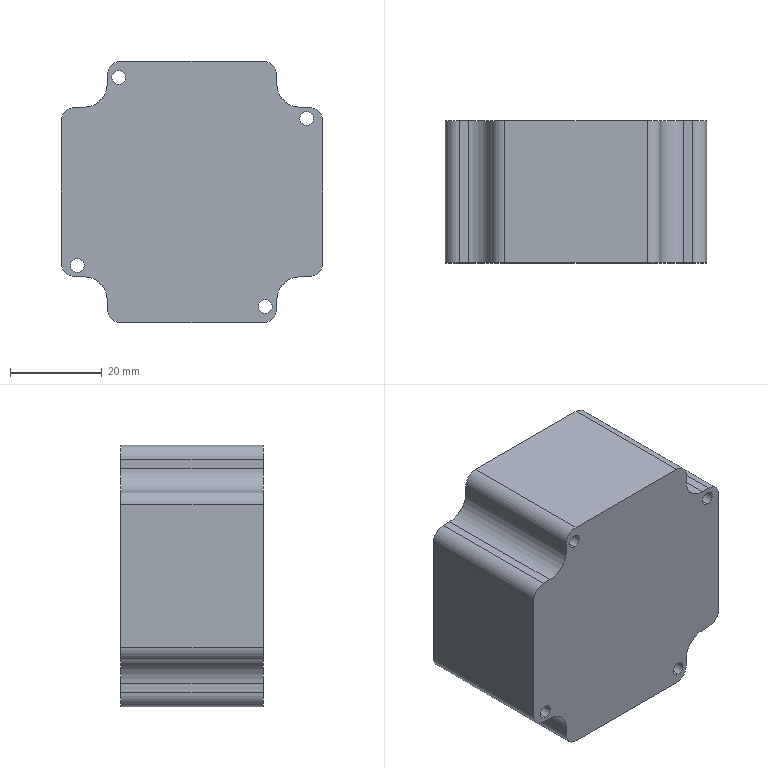Part | SolidWorks | features BaseBody 1 | 1 solid | 34 faces | box 57 x 31 x 57 mm | volume 87629 mm3 | cylinder 20 | plane 14 | commonest cylinder face diameters 3 x8 6 x8 10 x4
STEP:
#1=CARTESIAN_POINT('',(-16.,0.,23.5));
#2=VERTEX_POINT('',#1);
#3=CARTESIAN_POINT('',(-16.,0.,26.5));
#4=VERTEX_POINT('',#3);
#5=CARTESIAN_POINT('',(-16.,0.,25.));
#6=DIRECTION('',(0.,1.,0.));
#7=DIRECTION('',(0.,0.,1.));
#8=AXIS2_PLACEMENT_3D('',#5,#6,#7);
#9=CIRCLE('',#8,1.5);
#10=EDGE_CURVE('',#2,#4,#9,.T.);
#11=ORIENTED_EDGE('',*,*,#10,.F.);
#12=CARTESIAN_POINT('',(-16.,31.,23.5));
#13=VERTEX_POINT('',#12);
#14=CARTESIAN_POINT('',(-16.,0.,23.5));
#15=DIRECTION('',(0.,1.,0.));
#16=VECTOR('',#15,1000.);
#17=LINE('',#14,#16);
#18=EDGE_CURVE('',#2,#13,#17,.T.);
#19=ORIENTED_EDGE('',*,*,#18,.T.);
#20=CARTESIAN_POINT('',(-16.,31.,26.5));
#21=VERTEX_POINT('',#20);
#22=CARTESIAN_POINT('',(-16.,31.,25.));
#23=DIRECTION('',(0.,1.,0.));
#24=DIRECTION('',(0.,0.,1.));
#25=AXIS2_PLACEMENT_3D('',#22,#23,#24);
#26=CIRCLE('',#25,1.5);
#27=EDGE_CURVE('',#13,#21,#26,.T.);
#28=ORIENTED_EDGE('',*,*,#27,.T.);
#29=CARTESIAN_POINT('',(-16.,0.,26.5));
#30=DIRECTION('',(0.,1.,0.));
#31=VECTOR('',#30,1000.);
#32=LINE('',#29,#31);
#33=EDGE_CURVE('',#4,#21,#32,.T.);
#34=ORIENTED_EDGE('',*,*,#33,.F.);
#35=EDGE_LOOP('',(#11,#19,#28,#34));
#36=FACE_OUTER_BOUND('',#35,.T.);
#37=CARTESIAN_POINT('',(-16.,0.,25.));
#38=DIRECTION('',(0.,1.,0.));
#39=DIRECTION('',(0.,0.,1.));
#40=AXIS2_PLACEMENT_3D('',#37,#38,#39);
#41=CYLINDRICAL_SURFACE('',#40,1.5);
#42=ADVANCED_FACE('',(#36),#41,.F.);
#43=CARTESIAN_POINT('',(-25.,0.,-17.5));
#44=VERTEX_POINT('',#43);
#45=CARTESIAN_POINT('',(-25.,0.,-14.5));
#46=VERTEX_POINT('',#45);
#47=CARTESIAN_POINT('',(-25.,0.,-16.));
#48=DIRECTION('',(0.,1.,0.));
#49=DIRECTION('',(0.,0.,1.));
#50=AXIS2_PLACEMENT_3D('',#47,#48,#49);
#51=CIRCLE('',#50,1.5);
#52=EDGE_CURVE('',#44,#46,#51,.T.);
#53=ORIENTED_EDGE('',*,*,#52,.F.);
#54=CARTESIAN_POINT('',(-25.,31.,-17.5));
#55=VERTEX_POINT('',#54);
#56=CARTESIAN_POINT('',(-25.,0.,-17.5));
#57=DIRECTION('',(0.,1.,0.));
#58=VECTOR('',#57,1000.);
#59=LINE('',#56,#58);
#60=EDGE_CURVE('',#44,#55,#59,.T.);
#61=ORIENTED_EDGE('',*,*,#60,.T.);
#62=CARTESIAN_POINT('',(-25.,31.,-14.5));
#63=VERTEX_POINT('',#62);
#64=CARTESIAN_POINT('',(-25.,31.,-16.));
#65=DIRECTION('',(0.,1.,0.));
#66=DIRECTION('',(0.,0.,1.));
#67=AXIS2_PLACEMENT_3D('',#64,#65,#66);
#68=CIRCLE('',#67,1.5);
#69=EDGE_CURVE('',#55,#63,#68,.T.);
#70=ORIENTED_EDGE('',*,*,#69,.T.);
#71=CARTESIAN_POINT('',(-25.,0.,-14.5));
#72=DIRECTION('',(0.,1.,0.));
#73=VECTOR('',#72,1000.);
#74=LINE('',#71,#73);
#75=EDGE_CURVE('',#46,#63,#74,.T.);
#76=ORIENTED_EDGE('',*,*,#75,.F.);
#77=EDGE_LOOP('',(#53,#61,#70,#76));
#78=FACE_OUTER_BOUND('',#77,.T.);
#79=CARTESIAN_POINT('',(-25.,0.,-16.));
#80=DIRECTION('',(0.,1.,0.));
#81=DIRECTION('',(0.,0.,1.));
#82=AXIS2_PLACEMENT_3D('',#79,#80,#81);
#83=CYLINDRICAL_SURFACE('',#82,1.5);
#84=ADVANCED_FACE('',(#78),#83,.F.);
#85=CARTESIAN_POINT('',(16.,0.,-26.5));
#86=VERTEX_POINT('',#85);
#87=CARTESIAN_POINT('',(16.,0.,-23.5));
#88=VERTEX_POINT('',#87);
#89=CARTESIAN_POINT('',(16.,0.,-25.));
#90=DIRECTION('',(0.,1.,0.));
#91=DIRECTION('',(0.,0.,1.));
#92=AXIS2_PLACEMENT_3D('',#89,#90,#91);
#93=CIRCLE('',#92,1.5);
#94=EDGE_CURVE('',#86,#88,#93,.T.);
#95=ORIENTED_EDGE('',*,*,#94,.F.);
#96=CARTESIAN_POINT('',(16.,31.,-26.5));
#97=VERTEX_POINT('',#96);
#98=CARTESIAN_POINT('',(16.,0.,-26.5));
#99=DIRECTION('',(0.,1.,0.));
#100=VECTOR('',#99,1000.);
#101=LINE('',#98,#100);
#102=EDGE_CURVE('',#86,#97,#101,.T.);
#103=ORIENTED_EDGE('',*,*,#102,.T.);
#104=CARTESIAN_POINT('',(16.,31.,-23.5));
#105=VERTEX_POINT('',#104);
#106=CARTESIAN_POINT('',(16.,31.,-25.));
#107=DIRECTION('',(0.,1.,0.));
#108=DIRECTION('',(0.,0.,1.));
#109=AXIS2_PLACEMENT_3D('',#106,#107,#108);
#110=CIRCLE('',#109,1.5);
#111=EDGE_CURVE('',#97,#105,#110,.T.);
#112=ORIENTED_EDGE('',*,*,#111,.T.);
#113=CARTESIAN_POINT('',(16.,0.,-23.5));
#114=DIRECTION('',(0.,1.,0.));
#115=VECTOR('',#114,1000.);
#116=LINE('',#113,#115);
#117=EDGE_CURVE('',#88,#105,#116,.T.);
#118=ORIENTED_EDGE('',*,*,#117,.F.);
#119=EDGE_LOOP('',(#95,#103,#112,#118));
#120=FACE_OUTER_BOUND('',#119,.T.);
#121=CARTESIAN_POINT('',(16.,0.,-25.));
#122=DIRECTION('',(0.,1.,0.));
#123=DIRECTION('',(0.,0.,1.));
#124=AXIS2_PLACEMENT_3D('',#121,#122,#123);
#125=CYLINDRICAL_SURFACE('',#124,1.5);
#126=ADVANCED_FACE('',(#120),#125,.F.);
#127=CARTESIAN_POINT('',(25.,0.,14.5));
#128=VERTEX_POINT('',#127);
#129=CARTESIAN_POINT('',(25.,0.,17.5));
#130=VERTEX_POINT('',#129);
#131=CARTESIAN_POINT('',(25.,0.,16.));
#132=DIRECTION('',(0.,1.,0.));
#133=DIRECTION('',(0.,0.,1.));
#134=AXIS2_PLACEMENT_3D('',#131,#132,#133);
#135=CIRCLE('',#134,1.5);
#136=EDGE_CURVE('',#128,#130,#135,.T.);
#137=ORIENTED_EDGE('',*,*,#136,.F.);
#138=CARTESIAN_POINT('',(25.,31.,14.5));
#139=VERTEX_POINT('',#138);
#140=CARTESIAN_POINT('',(25.,0.,14.5));
#141=DIRECTION('',(0.,1.,0.));
#142=VECTOR('',#141,1000.);
#143=LINE('',#140,#142);
#144=EDGE_CURVE('',#128,#139,#143,.T.);
#145=ORIENTED_EDGE('',*,*,#144,.T.);
#146=CARTESIAN_POINT('',(25.,31.,17.5));
#147=VERTEX_POINT('',#146);
#148=CARTESIAN_POINT('',(25.,31.,16.));
#149=DIRECTION('',(0.,1.,0.));
#150=DIRECTION('',(0.,0.,1.));
#151=AXIS2_PLACEMENT_3D('',#148,#149,#150);
#152=CIRCLE('',#151,1.5);
#153=EDGE_CURVE('',#139,#147,#152,.T.);
#154=ORIENTED_EDGE('',*,*,#153,.T.);
#155=CARTESIAN_POINT('',(25.,0.,17.5));
#156=DIRECTION('',(0.,1.,0.));
#157=VECTOR('',#156,1000.);
#158=LINE('',#155,#157);
#159=EDGE_CURVE('',#130,#147,#158,.T.);
#160=ORIENTED_EDGE('',*,*,#159,.F.);
#161=EDGE_LOOP('',(#137,#145,#154,#160));
#162=FACE_OUTER_BOUND('',#161,.T.);
#163=CARTESIAN_POINT('',(25.,0.,16.));
#164=DIRECTION('',(0.,1.,0.));
#165=DIRECTION('',(0.,0.,1.));
#166=AXIS2_PLACEMENT_3D('',#163,#164,#165);
#167=CYLINDRICAL_SURFACE('',#166,1.5);
#168=ADVANCED_FACE('',(#162),#167,.F.);
#169=CARTESIAN_POINT('',(-16.,31.,25.));
#170=DIRECTION('',(0.,1.,0.));
#171=DIRECTION('',(0.,0.,1.));
#172=AXIS2_PLACEMENT_3D('',#169,#170,#171);
#173=CIRCLE('',#172,1.5);
#174=EDGE_CURVE('',#21,#13,#173,.T.);
#175=ORIENTED_EDGE('',*,*,#174,.F.);
#176=ORIENTED_EDGE('',*,*,#27,.F.);
#177=EDGE_LOOP('',(#175,#176));
#178=FACE_BOUND('',#177,.T.);
#179=CARTESIAN_POINT('',(-25.,31.,-16.));
#180=DIRECTION('',(0.,1.,0.));
#181=DIRECTION('',(0.,0.,1.));
#182=AXIS2_PLACEMENT_3D('',#179,#180,#181);
#183=CIRCLE('',#182,1.5);
#184=EDGE_CURVE('',#63,#55,#183,.T.);
#185=ORIENTED_EDGE('',*,*,#184,.F.);
#186=ORIENTED_EDGE('',*,*,#69,.F.);
#187=EDGE_LOOP('',(#185,#186));
#188=FACE_BOUND('',#187,.T.);
#189=CARTESIAN_POINT('',(16.,31.,-25.));
#190=DIRECTION('',(0.,1.,0.));
#191=DIRECTION('',(0.,0.,1.));
#192=AXIS2_PLACEMENT_3D('',#189,#190,#191);
#193=CIRCLE('',#192,1.5);
#194=EDGE_CURVE('',#105,#97,#193,.T.);
#195=ORIENTED_EDGE('',*,*,#194,.F.);
#196=ORIENTED_EDGE('',*,*,#111,.F.);
#197=EDGE_LOOP('',(#195,#196));
#198=FACE_BOUND('',#197,.T.);
#199=CARTESIAN_POINT('',(25.,31.,16.));
#200=DIRECTION('',(0.,1.,0.));
#201=DIRECTION('',(0.,0.,1.));
#202=AXIS2_PLACEMENT_3D('',#199,#200,#201);
#203=CIRCLE('',#202,1.5);
#204=EDGE_CURVE('',#147,#139,#203,.T.);
#205=ORIENTED_EDGE('',*,*,#204,.F.);
#206=ORIENTED_EDGE('',*,*,#153,.F.);
#207=EDGE_LOOP('',(#205,#206));
#208=FACE_BOUND('',#207,.T.);
#209=CARTESIAN_POINT('',(-18.5,31.,25.5));
#210=VERTEX_POINT('',#209);
#211=CARTESIAN_POINT('',(-18.5,31.,23.5));
#212=VERTEX_POINT('',#211);
#213=CARTESIAN_POINT('',(-18.5,31.,23.5));
#214=DIRECTION('',(0.,0.,-1.));
#215=VECTOR('',#214,1000.);
#216=LINE('',#213,#215);
#217=EDGE_CURVE('',#210,#212,#216,.T.);
#218=ORIENTED_EDGE('',*,*,#217,.F.);
#219=CARTESIAN_POINT('',(-15.5,31.,28.5));
#220=VERTEX_POINT('',#219);
#221=CARTESIAN_POINT('',(-15.5,31.,25.5));
#222=DIRECTION('',(0.,-1.,0.));
#223=DIRECTION('',(0.,0.,-1.));
#224=AXIS2_PLACEMENT_3D('',#221,#222,#223);
#225=CIRCLE('',#224,3.);
#226=EDGE_CURVE('',#220,#210,#225,.T.);
#227=ORIENTED_EDGE('',*,*,#226,.F.);
#228=CARTESIAN_POINT('',(15.5,31.,28.5));
#229=VERTEX_POINT('',#228);
#230=CARTESIAN_POINT('',(-23.5,31.,28.5));
#231=DIRECTION('',(-1.,0.,0.));
#232=VECTOR('',#231,1000.);
#233=LINE('',#230,#232);
#234=EDGE_CURVE('',#229,#220,#233,.T.);
#235=ORIENTED_EDGE('',*,*,#234,.F.);
#236=CARTESIAN_POINT('',(18.5,31.,25.5));
#237=VERTEX_POINT('',#236);
#238=CARTESIAN_POINT('',(15.5,31.,25.5));
#239=DIRECTION('',(0.,-1.,0.));
#240=DIRECTION('',(0.,0.,-1.));
#241=AXIS2_PLACEMENT_3D('',#238,#239,#240);
#242=CIRCLE('',#241,3.);
#243=EDGE_CURVE('',#237,#229,#242,.T.);
#244=ORIENTED_EDGE('',*,*,#243,.F.);
#245=CARTESIAN_POINT('',(18.5,31.,23.5));
#246=VERTEX_POINT('',#245);
#247=CARTESIAN_POINT('',(18.5,31.,23.5));
#248=DIRECTION('',(0.,0.,1.));
#249=VECTOR('',#248,1000.);
#250=LINE('',#247,#249);
#251=EDGE_CURVE('',#246,#237,#250,.T.);
#252=ORIENTED_EDGE('',*,*,#251,.F.);
#253=CARTESIAN_POINT('',(23.5,31.,18.5));
#254=VERTEX_POINT('',#253);
#255=CARTESIAN_POINT('',(23.5,31.,23.5));
#256=DIRECTION('',(0.,1.,0.));
#257=DIRECTION('',(0.,0.,-1.));
#258=AXIS2_PLACEMENT_3D('',#255,#256,#257);
#259=CIRCLE('',#258,5.);
#260=EDGE_CURVE('',#254,#246,#259,.T.);
#261=ORIENTED_EDGE('',*,*,#260,.F.);
#262=CARTESIAN_POINT('',(25.5,31.,18.5));
#263=VERTEX_POINT('',#262);
#264=CARTESIAN_POINT('',(-23.5,31.,18.5));
#265=DIRECTION('',(-1.,0.,0.));
#266=VECTOR('',#265,1000.);
#267=LINE('',#264,#266);
#268=EDGE_CURVE('',#263,#254,#267,.T.);
#269=ORIENTED_EDGE('',*,*,#268,.F.);
#270=CARTESIAN_POINT('',(28.5,31.,15.5));
#271=VERTEX_POINT('',#270);
#272=CARTESIAN_POINT('',(25.5,31.,15.5));
#273=DIRECTION('',(0.,-1.,0.));
#274=DIRECTION('',(0.,0.,-1.));
#275=AXIS2_PLACEMENT_3D('',#272,#273,#274);
#276=CIRCLE('',#275,3.);
#277=EDGE_CURVE('',#271,#263,#276,.T.);
#278=ORIENTED_EDGE('',*,*,#277,.F.);
#279=CARTESIAN_POINT('',(28.5,31.,-15.5));
#280=VERTEX_POINT('',#279);
#281=CARTESIAN_POINT('',(28.5,31.,23.5));
#282=DIRECTION('',(0.,0.,1.));
#283=VECTOR('',#282,1000.);
#284=LINE('',#281,#283);
#285=EDGE_CURVE('',#280,#271,#284,.T.);
#286=ORIENTED_EDGE('',*,*,#285,.F.);
#287=CARTESIAN_POINT('',(25.5,31.,-18.5));
#288=VERTEX_POINT('',#287);
#289=CARTESIAN_POINT('',(25.5,31.,-15.5));
#290=DIRECTION('',(0.,-1.,0.));
#291=DIRECTION('',(0.,0.,-1.));
#292=AXIS2_PLACEMENT_3D('',#289,#290,#291);
#293=CIRCLE('',#292,3.);
#294=EDGE_CURVE('',#288,#280,#293,.T.);
#295=ORIENTED_EDGE('',*,*,#294,.F.);
#296=CARTESIAN_POINT('',(23.5,31.,-18.5));
#297=VERTEX_POINT('',#296);
#298=CARTESIAN_POINT('',(-23.5,31.,-18.5));
#299=DIRECTION('',(1.,0.,0.));
#300=VECTOR('',#299,1000.);
#301=LINE('',#298,#300);
#302=EDGE_CURVE('',#297,#288,#301,.T.);
#303=ORIENTED_EDGE('',*,*,#302,.F.);
#304=CARTESIAN_POINT('',(18.5,31.,-23.5));
#305=VERTEX_POINT('',#304);
#306=CARTESIAN_POINT('',(23.5,31.,-23.5));
#307=DIRECTION('',(0.,1.,0.));
#308=DIRECTION('',(0.,0.,-1.));
#309=AXIS2_PLACEMENT_3D('',#306,#307,#308);
#310=CIRCLE('',#309,5.);
#311=EDGE_CURVE('',#305,#297,#310,.T.);
#312=ORIENTED_EDGE('',*,*,#311,.F.);
#313=CARTESIAN_POINT('',(18.5,31.,-25.5));
#314=VERTEX_POINT('',#313);
#315=CARTESIAN_POINT('',(18.5,31.,23.5));
#316=DIRECTION('',(0.,0.,1.));
#317=VECTOR('',#316,1000.);
#318=LINE('',#315,#317);
#319=EDGE_CURVE('',#314,#305,#318,.T.);
#320=ORIENTED_EDGE('',*,*,#319,.F.);
#321=CARTESIAN_POINT('',(15.5,31.,-28.5));
#322=VERTEX_POINT('',#321);
#323=CARTESIAN_POINT('',(15.5,31.,-25.5));
#324=DIRECTION('',(0.,-1.,0.));
#325=DIRECTION('',(0.,0.,-1.));
#326=AXIS2_PLACEMENT_3D('',#323,#324,#325);
#327=CIRCLE('',#326,3.);
#328=EDGE_CURVE('',#322,#314,#327,.T.);
#329=ORIENTED_EDGE('',*,*,#328,.F.);
#330=CARTESIAN_POINT('',(-15.5,31.,-28.5));
#331=VERTEX_POINT('',#330);
#332=CARTESIAN_POINT('',(-23.5,31.,-28.5));
#333=DIRECTION('',(1.,0.,0.));
#334=VECTOR('',#333,1000.);
#335=LINE('',#332,#334);
#336=EDGE_CURVE('',#331,#322,#335,.T.);
#337=ORIENTED_EDGE('',*,*,#336,.F.);
#338=CARTESIAN_POINT('',(-18.5,31.,-25.5));
#339=VERTEX_POINT('',#338);
#340=CARTESIAN_POINT('',(-15.5,31.,-25.5));
#341=DIRECTION('',(0.,-1.,0.));
#342=DIRECTION('',(0.,0.,-1.));
#343=AXIS2_PLACEMENT_3D('',#340,#341,#342);
#344=CIRCLE('',#343,3.);
#345=EDGE_CURVE('',#339,#331,#344,.T.);
#346=ORIENTED_EDGE('',*,*,#345,.F.);
#347=CARTESIAN_POINT('',(-18.5,31.,-23.5));
#348=VERTEX_POINT('',#347);
#349=CARTESIAN_POINT('',(-18.5,31.,23.5));
#350=DIRECTION('',(0.,0.,-1.));
#351=VECTOR('',#350,1000.);
#352=LINE('',#349,#351);
#353=EDGE_CURVE('',#348,#339,#352,.T.);
#354=ORIENTED_EDGE('',*,*,#353,.F.);
#355=CARTESIAN_POINT('',(-23.5,31.,-18.5));
#356=VERTEX_POINT('',#355);
#357=CARTESIAN_POINT('',(-23.5,31.,-23.5));
#358=DIRECTION('',(0.,1.,0.));
#359=DIRECTION('',(0.,0.,-1.));
#360=AXIS2_PLACEMENT_3D('',#357,#358,#359);
#361=CIRCLE('',#360,5.);
#362=EDGE_CURVE('',#356,#348,#361,.T.);
#363=ORIENTED_EDGE('',*,*,#362,.F.);
#364=CARTESIAN_POINT('',(-25.5,31.,-18.5));
#365=VERTEX_POINT('',#364);
#366=CARTESIAN_POINT('',(-23.5,31.,-18.5));
#367=DIRECTION('',(1.,0.,0.));
#368=VECTOR('',#367,1000.);
#369=LINE('',#366,#368);
#370=EDGE_CURVE('',#365,#356,#369,.T.);
#371=ORIENTED_EDGE('',*,*,#370,.F.);
#372=CARTESIAN_POINT('',(-28.5,31.,-15.5));
#373=VERTEX_POINT('',#372);
#374=CARTESIAN_POINT('',(-25.5,31.,-15.5));
#375=DIRECTION('',(0.,-1.,0.));
#376=DIRECTION('',(0.,0.,-1.));
#377=AXIS2_PLACEMENT_3D('',#374,#375,#376);
#378=CIRCLE('',#377,3.);
#379=EDGE_CURVE('',#373,#365,#378,.T.);
#380=ORIENTED_EDGE('',*,*,#379,.F.);
#381=CARTESIAN_POINT('',(-28.5,31.,15.5));
#382=VERTEX_POINT('',#381);
#383=CARTESIAN_POINT('',(-28.5,31.,23.5));
#384=DIRECTION('',(0.,0.,-1.));
#385=VECTOR('',#384,1000.);
#386=LINE('',#383,#385);
#387=EDGE_CURVE('',#382,#373,#386,.T.);
#388=ORIENTED_EDGE('',*,*,#387,.F.);
#389=CARTESIAN_POINT('',(-25.5,31.,18.5));
#390=VERTEX_POINT('',#389);
#391=CARTESIAN_POINT('',(-25.5,31.,15.5));
#392=DIRECTION('',(0.,-1.,0.));
#393=DIRECTION('',(0.,0.,-1.));
#394=AXIS2_PLACEMENT_3D('',#391,#392,#393);
#395=CIRCLE('',#394,3.);
#396=EDGE_CURVE('',#390,#382,#395,.T.);
#397=ORIENTED_EDGE('',*,*,#396,.F.);
#398=CARTESIAN_POINT('',(-23.5,31.,18.5));
#399=VERTEX_POINT('',#398);
#400=CARTESIAN_POINT('',(-23.5,31.,18.5));
#401=DIRECTION('',(-1.,0.,0.));
#402=VECTOR('',#401,1000.);
#403=LINE('',#400,#402);
#404=EDGE_CURVE('',#399,#390,#403,.T.);
#405=ORIENTED_EDGE('',*,*,#404,.F.);
#406=CARTESIAN_POINT('',(-23.5,31.,23.5));
#407=DIRECTION('',(0.,1.,0.));
#408=DIRECTION('',(0.,0.,-1.));
#409=AXIS2_PLACEMENT_3D('',#406,#407,#408);
#410=CIRCLE('',#409,5.);
#411=EDGE_CURVE('',#212,#399,#410,.T.);
#412=ORIENTED_EDGE('',*,*,#411,.F.);
#413=EDGE_LOOP('',(#218,#227,#235,#244,#252,#261,#269,#278,#286,#295,#303,#312,#320,#329,#337,#346,#354,#363,#371,#380,#388,#397,#405,#412));
#414=FACE_OUTER_BOUND('',#413,.T.);
#415=CARTESIAN_POINT('',(-23.5,31.,23.5));
#416=DIRECTION('',(0.,-1.,0.));
#417=DIRECTION('',(0.,0.,-1.));
#418=AXIS2_PLACEMENT_3D('',#415,#416,#417);
#419=PLANE('',#418);
#420=ADVANCED_FACE('',(#178,#188,#198,#208,#414),#419,.F.);
#421=CARTESIAN_POINT('',(-18.5,0.,23.5));
#422=VERTEX_POINT('',#421);
#423=CARTESIAN_POINT('',(-18.5,30.,23.5));
#424=DIRECTION('',(0.,-1.,0.));
#425=VECTOR('',#424,1000.);
#426=LINE('',#423,#425);
#427=EDGE_CURVE('',#212,#422,#426,.T.);
#428=ORIENTED_EDGE('',*,*,#427,.F.);
#429=ORIENTED_EDGE('',*,*,#411,.T.);
#430=CARTESIAN_POINT('',(-23.5,0.,18.5));
#431=VERTEX_POINT('',#430);
#432=CARTESIAN_POINT('',(-23.5,30.,18.5));
#433=DIRECTION('',(0.,1.,0.));
#434=VECTOR('',#433,1000.);
#435=LINE('',#432,#434);
#436=EDGE_CURVE('',#431,#399,#435,.T.);
#437=ORIENTED_EDGE('',*,*,#436,.F.);
#438=CARTESIAN_POINT('',(-23.5,0.,23.5));
#439=DIRECTION('',(0.,1.,0.));
#440=DIRECTION('',(0.,0.,-1.));
#441=AXIS2_PLACEMENT_3D('',#438,#439,#440);
#442=CIRCLE('',#441,5.);
#443=EDGE_CURVE('',#422,#431,#442,.T.);
#444=ORIENTED_EDGE('',*,*,#443,.F.);
#445=EDGE_LOOP('',(#428,#429,#437,#444));
#446=FACE_OUTER_BOUND('',#445,.T.);
#447=CARTESIAN_POINT('',(-23.5,30.,23.5));
#448=DIRECTION('',(0.,-1.,0.));
#449=DIRECTION('',(0.,0.,-1.));
#450=AXIS2_PLACEMENT_3D('',#447,#448,#449);
#451=CYLINDRICAL_SURFACE('',#450,5.);
#452=ADVANCED_FACE('',(#446),#451,.F.);
#453=CARTESIAN_POINT('',(-18.5,0.,25.5));
#454=VERTEX_POINT('',#453);
#455=CARTESIAN_POINT('',(-18.5,30.,25.5));
#456=DIRECTION('',(0.,-1.,0.));
#457=VECTOR('',#456,1000.);
#458=LINE('',#455,#457);
#459=EDGE_CURVE('',#210,#454,#458,.T.);
#460=ORIENTED_EDGE('',*,*,#459,.F.);
#461=ORIENTED_EDGE('',*,*,#217,.T.);
#462=ORIENTED_EDGE('',*,*,#427,.T.);
#463=CARTESIAN_POINT('',(-18.5,0.,23.5));
#464=DIRECTION('',(0.,0.,-1.));
#465=VECTOR('',#464,1000.);
#466=LINE('',#463,#465);
#467=EDGE_CURVE('',#454,#422,#466,.T.);
#468=ORIENTED_EDGE('',*,*,#467,.F.);
#469=EDGE_LOOP('',(#460,#461,#462,#468));
#470=FACE_OUTER_BOUND('',#469,.T.);
#471=CARTESIAN_POINT('',(-18.5,30.,23.5));
#472=DIRECTION('',(1.,0.,0.));
#473=DIRECTION('',(0.,1.,0.));
#474=AXIS2_PLACEMENT_3D('',#471,#472,#473);
#475=PLANE('',#474);
#476=ADVANCED_FACE('',(#470),#475,.F.);
#477=ORIENTED_EDGE('',*,*,#226,.T.);
#478=ORIENTED_EDGE('',*,*,#459,.T.);
#479=CARTESIAN_POINT('',(-15.5,0.,28.5));
#480=VERTEX_POINT('',#479);
#481=CARTESIAN_POINT('',(-15.5,0.,25.5));
#482=DIRECTION('',(0.,1.,0.));
#483=DIRECTION('',(0.,0.,-1.));
#484=AXIS2_PLACEMENT_3D('',#481,#482,#483);
#485=CIRCLE('',#484,3.);
#486=EDGE_CURVE('',#454,#480,#485,.T.);
#487=ORIENTED_EDGE('',*,*,#486,.T.);
#488=CARTESIAN_POINT('',(-15.5,30.,28.5));
#489=DIRECTION('',(0.,1.,0.));
#490=VECTOR('',#489,1000.);
#491=LINE('',#488,#490);
#492=EDGE_CURVE('',#480,#220,#491,.T.);
#493=ORIENTED_EDGE('',*,*,#492,.T.);
#494=EDGE_LOOP('',(#477,#478,#487,#493));
#495=FACE_OUTER_BOUND('',#494,.T.);
#496=CARTESIAN_POINT('',(-15.5,30.,25.5));
#497=DIRECTION('',(0.,-1.,0.));
#498=DIRECTION('',(0.,0.,-1.));
#499=AXIS2_PLACEMENT_3D('',#496,#497,#498);
#500=CYLINDRICAL_SURFACE('',#499,3.);
#501=ADVANCED_FACE('',(#495),#500,.T.);
#502=CARTESIAN_POINT('',(15.5,0.,28.5));
#503=VERTEX_POINT('',#502);
#504=CARTESIAN_POINT('',(15.5,30.,28.5));
#505=DIRECTION('',(0.,-1.,0.));
#506=VECTOR('',#505,1000.);
#507=LINE('',#504,#506);
#508=EDGE_CURVE('',#229,#503,#507,.T.);
#509=ORIENTED_EDGE('',*,*,#508,.F.);
#510=ORIENTED_EDGE('',*,*,#234,.T.);
#511=ORIENTED_EDGE('',*,*,#492,.F.);
#512=CARTESIAN_POINT('',(-15.5,0.,28.5));
#513=DIRECTION('',(-1.,0.,0.));
#514=VECTOR('',#513,1000.);
#515=LINE('',#512,#514);
#516=EDGE_CURVE('',#503,#480,#515,.T.);
#517=ORIENTED_EDGE('',*,*,#516,.F.);
#518=EDGE_LOOP('',(#509,#510,#511,#517));
#519=FACE_OUTER_BOUND('',#518,.T.);
#520=CARTESIAN_POINT('',(-15.5,30.,28.5));
#521=DIRECTION('',(0.,0.,-1.));
#522=DIRECTION('',(0.,-1.,0.));
#523=AXIS2_PLACEMENT_3D('',#520,#521,#522);
#524=PLANE('',#523);
#525=ADVANCED_FACE('',(#519),#524,.F.);
#526=ORIENTED_EDGE('',*,*,#243,.T.);
#527=ORIENTED_EDGE('',*,*,#508,.T.);
#528=CARTESIAN_POINT('',(18.5,0.,25.5));
#529=VERTEX_POINT('',#528);
#530=CARTESIAN_POINT('',(15.5,0.,25.5));
#531=DIRECTION('',(0.,1.,0.));
#532=DIRECTION('',(0.,0.,-1.));
#533=AXIS2_PLACEMENT_3D('',#530,#531,#532);
#534=CIRCLE('',#533,3.);
#535=EDGE_CURVE('',#503,#529,#534,.T.);
#536=ORIENTED_EDGE('',*,*,#535,.T.);
#537=CARTESIAN_POINT('',(18.5,30.,25.5));
#538=DIRECTION('',(0.,1.,0.));
#539=VECTOR('',#538,1000.);
#540=LINE('',#537,#539);
#541=EDGE_CURVE('',#529,#237,#540,.T.);
#542=ORIENTED_EDGE('',*,*,#541,.T.);
#543=EDGE_LOOP('',(#526,#527,#536,#542));
#544=FACE_OUTER_BOUND('',#543,.T.);
#545=CARTESIAN_POINT('',(15.5,30.,25.5));
#546=DIRECTION('',(0.,-1.,0.));
#547=DIRECTION('',(0.,0.,-1.));
#548=AXIS2_PLACEMENT_3D('',#545,#546,#547);
#549=CYLINDRICAL_SURFACE('',#548,3.);
#550=ADVANCED_FACE('',(#544),#549,.T.);
#551=CARTESIAN_POINT('',(18.5,0.,23.5));
#552=VERTEX_POINT('',#551);
#553=CARTESIAN_POINT('',(18.5,30.,23.5));
#554=DIRECTION('',(0.,-1.,0.));
#555=VECTOR('',#554,1000.);
#556=LINE('',#553,#555);
#557=EDGE_CURVE('',#246,#552,#556,.T.);
#558=ORIENTED_EDGE('',*,*,#557,.F.);
#559=ORIENTED_EDGE('',*,*,#251,.T.);
#560=ORIENTED_EDGE('',*,*,#541,.F.);
#561=CARTESIAN_POINT('',(18.5,0.,25.5));
#562=DIRECTION('',(0.,0.,1.));
#563=VECTOR('',#562,1000.);
#564=LINE('',#561,#563);
#565=EDGE_CURVE('',#552,#529,#564,.T.);
#566=ORIENTED_EDGE('',*,*,#565,.F.);
#567=EDGE_LOOP('',(#558,#559,#560,#566));
#568=FACE_OUTER_BOUND('',#567,.T.);
#569=CARTESIAN_POINT('',(18.5,30.,25.5));
#570=DIRECTION('',(-1.,0.,0.));
#571=DIRECTION('',(0.,0.,1.));
#572=AXIS2_PLACEMENT_3D('',#569,#570,#571);
#573=PLANE('',#572);
#574=ADVANCED_FACE('',(#568),#573,.F.);
#575=CARTESIAN_POINT('',(23.5,0.,18.5));
#576=VERTEX_POINT('',#575);
#577=CARTESIAN_POINT('',(23.5,30.,18.5));
#578=DIRECTION('',(0.,-1.,0.));
#579=VECTOR('',#578,1000.);
#580=LINE('',#577,#579);
#581=EDGE_CURVE('',#254,#576,#580,.T.);
#582=ORIENTED_EDGE('',*,*,#581,.F.);
#583=ORIENTED_EDGE('',*,*,#260,.T.);
#584=ORIENTED_EDGE('',*,*,#557,.T.);
#585=CARTESIAN_POINT('',(23.5,0.,23.5));
#586=DIRECTION('',(0.,1.,0.));
#587=DIRECTION('',(0.,0.,-1.));
#588=AXIS2_PLACEMENT_3D('',#585,#586,#587);
#589=CIRCLE('',#588,5.);
#590=EDGE_CURVE('',#576,#552,#589,.T.);
#591=ORIENTED_EDGE('',*,*,#590,.F.);
#592=EDGE_LOOP('',(#582,#583,#584,#591));
#593=FACE_OUTER_BOUND('',#592,.T.);
#594=CARTESIAN_POINT('',(23.5,30.,23.5));
#595=DIRECTION('',(0.,-1.,0.));
#596=DIRECTION('',(0.,0.,-1.));
#597=AXIS2_PLACEMENT_3D('',#594,#595,#596);
#598=CYLINDRICAL_SURFACE('',#597,5.);
#599=ADVANCED_FACE('',(#593),#598,.F.);
#600=CARTESIAN_POINT('',(25.5,0.,18.5));
#601=VERTEX_POINT('',#600);
#602=CARTESIAN_POINT('',(25.5,30.,18.5));
#603=DIRECTION('',(0.,-1.,0.));
#604=VECTOR('',#603,1000.);
#605=LINE('',#602,#604);
#606=EDGE_CURVE('',#263,#601,#605,.T.);
#607=ORIENTED_EDGE('',*,*,#606,.F.);
#608=ORIENTED_EDGE('',*,*,#268,.T.);
#609=ORIENTED_EDGE('',*,*,#581,.T.);
#610=CARTESIAN_POINT('',(23.5,0.,18.5));
#611=DIRECTION('',(-1.,0.,0.));
#612=VECTOR('',#611,1000.);
#613=LINE('',#610,#612);
#614=EDGE_CURVE('',#601,#576,#613,.T.);
#615=ORIENTED_EDGE('',*,*,#614,.F.);
#616=EDGE_LOOP('',(#607,#608,#609,#615));
#617=FACE_OUTER_BOUND('',#616,.T.);
#618=CARTESIAN_POINT('',(23.5,30.,18.5));
#619=DIRECTION('',(0.,0.,-1.));
#620=DIRECTION('',(0.,-1.,0.));
#621=AXIS2_PLACEMENT_3D('',#618,#619,#620);
#622=PLANE('',#621);
#623=ADVANCED_FACE('',(#617),#622,.F.);
#624=ORIENTED_EDGE('',*,*,#277,.T.);
#625=ORIENTED_EDGE('',*,*,#606,.T.);
#626=CARTESIAN_POINT('',(28.5,0.,15.5));
#627=VERTEX_POINT('',#626);
#628=CARTESIAN_POINT('',(25.5,0.,15.5));
#629=DIRECTION('',(0.,1.,0.));
#630=DIRECTION('',(0.,0.,-1.));
#631=AXIS2_PLACEMENT_3D('',#628,#629,#630);
#632=CIRCLE('',#631,3.);
#633=EDGE_CURVE('',#601,#627,#632,.T.);
#634=ORIENTED_EDGE('',*,*,#633,.T.);
#635=CARTESIAN_POINT('',(28.5,30.,15.5));
#636=DIRECTION('',(0.,1.,0.));
#637=VECTOR('',#636,1000.);
#638=LINE('',#635,#637);
#639=EDGE_CURVE('',#627,#271,#638,.T.);
#640=ORIENTED_EDGE('',*,*,#639,.T.);
#641=EDGE_LOOP('',(#624,#625,#634,#640));
#642=FACE_OUTER_BOUND('',#641,.T.);
#643=CARTESIAN_POINT('',(25.5,30.,15.5));
#644=DIRECTION('',(0.,-1.,0.));
#645=DIRECTION('',(0.,0.,-1.));
#646=AXIS2_PLACEMENT_3D('',#643,#644,#645);
#647=CYLINDRICAL_SURFACE('',#646,3.);
#648=ADVANCED_FACE('',(#642),#647,.T.);
#649=CARTESIAN_POINT('',(28.5,0.,-15.5));
#650=VERTEX_POINT('',#649);
#651=CARTESIAN_POINT('',(28.5,30.,-15.5));
#652=DIRECTION('',(0.,-1.,0.));
#653=VECTOR('',#652,1000.);
#654=LINE('',#651,#653);
#655=EDGE_CURVE('',#280,#650,#654,.T.);
#656=ORIENTED_EDGE('',*,*,#655,.F.);
#657=ORIENTED_EDGE('',*,*,#285,.T.);
#658=ORIENTED_EDGE('',*,*,#639,.F.);
#659=CARTESIAN_POINT('',(28.5,0.,15.5));
#660=DIRECTION('',(0.,0.,1.));
#661=VECTOR('',#660,1000.);
#662=LINE('',#659,#661);
#663=EDGE_CURVE('',#650,#627,#662,.T.);
#664=ORIENTED_EDGE('',*,*,#663,.F.);
#665=EDGE_LOOP('',(#656,#657,#658,#664));
#666=FACE_OUTER_BOUND('',#665,.T.);
#667=CARTESIAN_POINT('',(28.5,30.,15.5));
#668=DIRECTION('',(-1.,0.,0.));
#669=DIRECTION('',(0.,1.,0.));
#670=AXIS2_PLACEMENT_3D('',#667,#668,#669);
#671=PLANE('',#670);
#672=ADVANCED_FACE('',(#666),#671,.F.);
#673=ORIENTED_EDGE('',*,*,#294,.T.);
#674=ORIENTED_EDGE('',*,*,#655,.T.);
#675=CARTESIAN_POINT('',(25.5,0.,-18.5));
#676=VERTEX_POINT('',#675);
#677=CARTESIAN_POINT('',(25.5,0.,-15.5));
#678=DIRECTION('',(0.,1.,0.));
#679=DIRECTION('',(0.,0.,-1.));
#680=AXIS2_PLACEMENT_3D('',#677,#678,#679);
#681=CIRCLE('',#680,3.);
#682=EDGE_CURVE('',#650,#676,#681,.T.);
#683=ORIENTED_EDGE('',*,*,#682,.T.);
#684=CARTESIAN_POINT('',(25.5,30.,-18.5));
#685=DIRECTION('',(0.,1.,0.));
#686=VECTOR('',#685,1000.);
#687=LINE('',#684,#686);
#688=EDGE_CURVE('',#676,#288,#687,.T.);
#689=ORIENTED_EDGE('',*,*,#688,.T.);
#690=EDGE_LOOP('',(#673,#674,#683,#689));
#691=FACE_OUTER_BOUND('',#690,.T.);
#692=CARTESIAN_POINT('',(25.5,30.,-15.5));
#693=DIRECTION('',(0.,-1.,0.));
#694=DIRECTION('',(0.,0.,-1.));
#695=AXIS2_PLACEMENT_3D('',#692,#693,#694);
#696=CYLINDRICAL_SURFACE('',#695,3.);
#697=ADVANCED_FACE('',(#691),#696,.T.);
#698=CARTESIAN_POINT('',(23.5,0.,-18.5));
#699=VERTEX_POINT('',#698);
#700=CARTESIAN_POINT('',(23.5,30.,-18.5));
#701=DIRECTION('',(0.,-1.,0.));
#702=VECTOR('',#701,1000.);
#703=LINE('',#700,#702);
#704=EDGE_CURVE('',#297,#699,#703,.T.);
#705=ORIENTED_EDGE('',*,*,#704,.F.);
#706=ORIENTED_EDGE('',*,*,#302,.T.);
#707=ORIENTED_EDGE('',*,*,#688,.F.);
#708=CARTESIAN_POINT('',(25.5,0.,-18.5));
#709=DIRECTION('',(1.,0.,0.));
#710=VECTOR('',#709,1000.);
#711=LINE('',#708,#710);
#712=EDGE_CURVE('',#699,#676,#711,.T.);
#713=ORIENTED_EDGE('',*,*,#712,.F.);
#714=EDGE_LOOP('',(#705,#706,#707,#713));
#715=FACE_OUTER_BOUND('',#714,.T.);
#716=CARTESIAN_POINT('',(25.5,30.,-18.5));
#717=DIRECTION('',(0.,0.,1.));
#718=DIRECTION('',(1.,0.,0.));
#719=AXIS2_PLACEMENT_3D('',#716,#717,#718);
#720=PLANE('',#719);
#721=ADVANCED_FACE('',(#715),#720,.F.);
#722=CARTESIAN_POINT('',(18.5,0.,-23.5));
#723=VERTEX_POINT('',#722);
#724=CARTESIAN_POINT('',(18.5,30.,-23.5));
#725=DIRECTION('',(0.,-1.,0.));
#726=VECTOR('',#725,1000.);
#727=LINE('',#724,#726);
#728=EDGE_CURVE('',#305,#723,#727,.T.);
#729=ORIENTED_EDGE('',*,*,#728,.F.);
#730=ORIENTED_EDGE('',*,*,#311,.T.);
#731=ORIENTED_EDGE('',*,*,#704,.T.);
#732=CARTESIAN_POINT('',(23.5,0.,-23.5));
#733=DIRECTION('',(0.,1.,0.));
#734=DIRECTION('',(0.,0.,-1.));
#735=AXIS2_PLACEMENT_3D('',#732,#733,#734);
#736=CIRCLE('',#735,5.);
#737=EDGE_CURVE('',#723,#699,#736,.T.);
#738=ORIENTED_EDGE('',*,*,#737,.F.);
#739=EDGE_LOOP('',(#729,#730,#731,#738));
#740=FACE_OUTER_BOUND('',#739,.T.);
#741=CARTESIAN_POINT('',(23.5,30.,-23.5));
#742=DIRECTION('',(0.,-1.,0.));
#743=DIRECTION('',(0.,0.,-1.));
#744=AXIS2_PLACEMENT_3D('',#741,#742,#743);
#745=CYLINDRICAL_SURFACE('',#744,5.);
#746=ADVANCED_FACE('',(#740),#745,.F.);
#747=CARTESIAN_POINT('',(18.5,0.,-25.5));
#748=VERTEX_POINT('',#747);
#749=CARTESIAN_POINT('',(18.5,30.,-25.5));
#750=DIRECTION('',(0.,-1.,0.));
#751=VECTOR('',#750,1000.);
#752=LINE('',#749,#751);
#753=EDGE_CURVE('',#314,#748,#752,.T.);
#754=ORIENTED_EDGE('',*,*,#753,.F.);
#755=ORIENTED_EDGE('',*,*,#319,.T.);
#756=ORIENTED_EDGE('',*,*,#728,.T.);
#757=CARTESIAN_POINT('',(18.5,0.,-23.5));
#758=DIRECTION('',(0.,0.,1.));
#759=VECTOR('',#758,1000.);
#760=LINE('',#757,#759);
#761=EDGE_CURVE('',#748,#723,#760,.T.);
#762=ORIENTED_EDGE('',*,*,#761,.F.);
#763=EDGE_LOOP('',(#754,#755,#756,#762));
#764=FACE_OUTER_BOUND('',#763,.T.);
#765=CARTESIAN_POINT('',(18.5,30.,-23.5));
#766=DIRECTION('',(-1.,0.,0.));
#767=DIRECTION('',(0.,0.,1.));
#768=AXIS2_PLACEMENT_3D('',#765,#766,#767);
#769=PLANE('',#768);
#770=ADVANCED_FACE('',(#764),#769,.F.);
#771=ORIENTED_EDGE('',*,*,#328,.T.);
#772=ORIENTED_EDGE('',*,*,#753,.T.);
#773=CARTESIAN_POINT('',(15.5,0.,-28.5));
#774=VERTEX_POINT('',#773);
#775=CARTESIAN_POINT('',(15.5,0.,-25.5));
#776=DIRECTION('',(0.,1.,0.));
#777=DIRECTION('',(0.,0.,-1.));
#778=AXIS2_PLACEMENT_3D('',#775,#776,#777);
#779=CIRCLE('',#778,3.);
#780=EDGE_CURVE('',#748,#774,#779,.T.);
#781=ORIENTED_EDGE('',*,*,#780,.T.);
#782=CARTESIAN_POINT('',(15.5,30.,-28.5));
#783=DIRECTION('',(0.,1.,0.));
#784=VECTOR('',#783,1000.);
#785=LINE('',#782,#784);
#786=EDGE_CURVE('',#774,#322,#785,.T.);
#787=ORIENTED_EDGE('',*,*,#786,.T.);
#788=EDGE_LOOP('',(#771,#772,#781,#787));
#789=FACE_OUTER_BOUND('',#788,.T.);
#790=CARTESIAN_POINT('',(15.5,30.,-25.5));
#791=DIRECTION('',(0.,-1.,0.));
#792=DIRECTION('',(0.,0.,-1.));
#793=AXIS2_PLACEMENT_3D('',#790,#791,#792);
#794=CYLINDRICAL_SURFACE('',#793,3.);
#795=ADVANCED_FACE('',(#789),#794,.T.);
#796=CARTESIAN_POINT('',(-15.5,0.,-28.5));
#797=VERTEX_POINT('',#796);
#798=CARTESIAN_POINT('',(-15.5,30.,-28.5));
#799=DIRECTION('',(0.,-1.,0.));
#800=VECTOR('',#799,1000.);
#801=LINE('',#798,#800);
#802=EDGE_CURVE('',#331,#797,#801,.T.);
#803=ORIENTED_EDGE('',*,*,#802,.F.);
#804=ORIENTED_EDGE('',*,*,#336,.T.);
#805=ORIENTED_EDGE('',*,*,#786,.F.);
#806=CARTESIAN_POINT('',(15.5,0.,-28.5));
#807=DIRECTION('',(1.,0.,0.));
#808=VECTOR('',#807,1000.);
#809=LINE('',#806,#808);
#810=EDGE_CURVE('',#797,#774,#809,.T.);
#811=ORIENTED_EDGE('',*,*,#810,.F.);
#812=EDGE_LOOP('',(#803,#804,#805,#811));
#813=FACE_OUTER_BOUND('',#812,.T.);
#814=CARTESIAN_POINT('',(15.5,30.,-28.5));
#815=DIRECTION('',(0.,0.,1.));
#816=DIRECTION('',(1.,0.,0.));
#817=AXIS2_PLACEMENT_3D('',#814,#815,#816);
#818=PLANE('',#817);
#819=ADVANCED_FACE('',(#813),#818,.F.);
#820=ORIENTED_EDGE('',*,*,#345,.T.);
#821=ORIENTED_EDGE('',*,*,#802,.T.);
#822=CARTESIAN_POINT('',(-18.5,0.,-25.5));
#823=VERTEX_POINT('',#822);
#824=CARTESIAN_POINT('',(-15.5,0.,-25.5));
#825=DIRECTION('',(0.,1.,0.));
#826=DIRECTION('',(0.,0.,-1.));
#827=AXIS2_PLACEMENT_3D('',#824,#825,#826);
#828=CIRCLE('',#827,3.);
#829=EDGE_CURVE('',#797,#823,#828,.T.);
#830=ORIENTED_EDGE('',*,*,#829,.T.);
#831=CARTESIAN_POINT('',(-18.5,30.,-25.5));
#832=DIRECTION('',(0.,1.,0.));
#833=VECTOR('',#832,1000.);
#834=LINE('',#831,#833);
#835=EDGE_CURVE('',#823,#339,#834,.T.);
#836=ORIENTED_EDGE('',*,*,#835,.T.);
#837=EDGE_LOOP('',(#820,#821,#830,#836));
#838=FACE_OUTER_BOUND('',#837,.T.);
#839=CARTESIAN_POINT('',(-15.5,30.,-25.5));
#840=DIRECTION('',(0.,-1.,0.));
#841=DIRECTION('',(0.,0.,-1.));
#842=AXIS2_PLACEMENT_3D('',#839,#840,#841);
#843=CYLINDRICAL_SURFACE('',#842,3.);
#844=ADVANCED_FACE('',(#838),#843,.T.);
#845=CARTESIAN_POINT('',(-18.5,0.,-23.5));
#846=VERTEX_POINT('',#845);
#847=CARTESIAN_POINT('',(-18.5,30.,-23.5));
#848=DIRECTION('',(0.,-1.,0.));
#849=VECTOR('',#848,1000.);
#850=LINE('',#847,#849);
#851=EDGE_CURVE('',#348,#846,#850,.T.);
#852=ORIENTED_EDGE('',*,*,#851,.F.);
#853=ORIENTED_EDGE('',*,*,#353,.T.);
#854=ORIENTED_EDGE('',*,*,#835,.F.);
#855=CARTESIAN_POINT('',(-18.5,0.,-25.5));
#856=DIRECTION('',(0.,0.,-1.));
#857=VECTOR('',#856,1000.);
#858=LINE('',#855,#857);
#859=EDGE_CURVE('',#846,#823,#858,.T.);
#860=ORIENTED_EDGE('',*,*,#859,.F.);
#861=EDGE_LOOP('',(#852,#853,#854,#860));
#862=FACE_OUTER_BOUND('',#861,.T.);
#863=CARTESIAN_POINT('',(-18.5,30.,-25.5));
#864=DIRECTION('',(1.,0.,0.));
#865=DIRECTION('',(0.,1.,0.));
#866=AXIS2_PLACEMENT_3D('',#863,#864,#865);
#867=PLANE('',#866);
#868=ADVANCED_FACE('',(#862),#867,.F.);
#869=CARTESIAN_POINT('',(-23.5,0.,-18.5));
#870=VERTEX_POINT('',#869);
#871=CARTESIAN_POINT('',(-23.5,30.,-18.5));
#872=DIRECTION('',(0.,-1.,0.));
#873=VECTOR('',#872,1000.);
#874=LINE('',#871,#873);
#875=EDGE_CURVE('',#356,#870,#874,.T.);
#876=ORIENTED_EDGE('',*,*,#875,.F.);
#877=ORIENTED_EDGE('',*,*,#362,.T.);
#878=ORIENTED_EDGE('',*,*,#851,.T.);
#879=CARTESIAN_POINT('',(-23.5,0.,-23.5));
#880=DIRECTION('',(0.,1.,0.));
#881=DIRECTION('',(0.,0.,-1.));
#882=AXIS2_PLACEMENT_3D('',#879,#880,#881);
#883=CIRCLE('',#882,5.);
#884=EDGE_CURVE('',#870,#846,#883,.T.);
#885=ORIENTED_EDGE('',*,*,#884,.F.);
#886=EDGE_LOOP('',(#876,#877,#878,#885));
#887=FACE_OUTER_BOUND('',#886,.T.);
#888=CARTESIAN_POINT('',(-23.5,30.,-23.5));
#889=DIRECTION('',(0.,-1.,0.));
#890=DIRECTION('',(0.,0.,-1.));
#891=AXIS2_PLACEMENT_3D('',#888,#889,#890);
#892=CYLINDRICAL_SURFACE('',#891,5.);
#893=ADVANCED_FACE('',(#887),#892,.F.);
#894=CARTESIAN_POINT('',(-25.5,0.,-18.5));
#895=VERTEX_POINT('',#894);
#896=CARTESIAN_POINT('',(-25.5,30.,-18.5));
#897=DIRECTION('',(0.,-1.,0.));
#898=VECTOR('',#897,1000.);
#899=LINE('',#896,#898);
#900=EDGE_CURVE('',#365,#895,#899,.T.);
#901=ORIENTED_EDGE('',*,*,#900,.F.);
#902=ORIENTED_EDGE('',*,*,#370,.T.);
#903=ORIENTED_EDGE('',*,*,#875,.T.);
#904=CARTESIAN_POINT('',(-23.5,0.,-18.5));
#905=DIRECTION('',(1.,0.,0.));
#906=VECTOR('',#905,1000.);
#907=LINE('',#904,#906);
#908=EDGE_CURVE('',#895,#870,#907,.T.);
#909=ORIENTED_EDGE('',*,*,#908,.F.);
#910=EDGE_LOOP('',(#901,#902,#903,#909));
#911=FACE_OUTER_BOUND('',#910,.T.);
#912=CARTESIAN_POINT('',(-23.5,30.,-18.5));
#913=DIRECTION('',(0.,0.,1.));
#914=DIRECTION('',(1.,0.,0.));
#915=AXIS2_PLACEMENT_3D('',#912,#913,#914);
#916=PLANE('',#915);
#917=ADVANCED_FACE('',(#911),#916,.F.);
#918=ORIENTED_EDGE('',*,*,#379,.T.);
#919=ORIENTED_EDGE('',*,*,#900,.T.);
#920=CARTESIAN_POINT('',(-28.5,0.,-15.5));
#921=VERTEX_POINT('',#920);
#922=CARTESIAN_POINT('',(-25.5,0.,-15.5));
#923=DIRECTION('',(0.,1.,0.));
#924=DIRECTION('',(0.,0.,-1.));
#925=AXIS2_PLACEMENT_3D('',#922,#923,#924);
#926=CIRCLE('',#925,3.);
#927=EDGE_CURVE('',#895,#921,#926,.T.);
#928=ORIENTED_EDGE('',*,*,#927,.T.);
#929=CARTESIAN_POINT('',(-28.5,30.,-15.5));
#930=DIRECTION('',(0.,1.,0.));
#931=VECTOR('',#930,1000.);
#932=LINE('',#929,#931);
#933=EDGE_CURVE('',#921,#373,#932,.T.);
#934=ORIENTED_EDGE('',*,*,#933,.T.);
#935=EDGE_LOOP('',(#918,#919,#928,#934));
#936=FACE_OUTER_BOUND('',#935,.T.);
#937=CARTESIAN_POINT('',(-25.5,30.,-15.5));
#938=DIRECTION('',(0.,-1.,0.));
#939=DIRECTION('',(0.,0.,-1.));
#940=AXIS2_PLACEMENT_3D('',#937,#938,#939);
#941=CYLINDRICAL_SURFACE('',#940,3.);
#942=ADVANCED_FACE('',(#936),#941,.T.);
#943=CARTESIAN_POINT('',(-28.5,0.,15.5));
#944=VERTEX_POINT('',#943);
#945=CARTESIAN_POINT('',(-28.5,30.,15.5));
#946=DIRECTION('',(0.,-1.,0.));
#947=VECTOR('',#946,1000.);
#948=LINE('',#945,#947);
#949=EDGE_CURVE('',#382,#944,#948,.T.);
#950=ORIENTED_EDGE('',*,*,#949,.F.);
#951=ORIENTED_EDGE('',*,*,#387,.T.);
#952=ORIENTED_EDGE('',*,*,#933,.F.);
#953=CARTESIAN_POINT('',(-28.5,0.,-15.5));
#954=DIRECTION('',(0.,0.,-1.));
#955=VECTOR('',#954,1000.);
#956=LINE('',#953,#955);
#957=EDGE_CURVE('',#944,#921,#956,.T.);
#958=ORIENTED_EDGE('',*,*,#957,.F.);
#959=EDGE_LOOP('',(#950,#951,#952,#958));
#960=FACE_OUTER_BOUND('',#959,.T.);
#961=CARTESIAN_POINT('',(-28.5,30.,-15.5));
#962=DIRECTION('',(1.,0.,0.));
#963=DIRECTION('',(0.,0.,-1.));
#964=AXIS2_PLACEMENT_3D('',#961,#962,#963);
#965=PLANE('',#964);
#966=ADVANCED_FACE('',(#960),#965,.F.);
#967=ORIENTED_EDGE('',*,*,#396,.T.);
#968=ORIENTED_EDGE('',*,*,#949,.T.);
#969=CARTESIAN_POINT('',(-25.5,0.,18.5));
#970=VERTEX_POINT('',#969);
#971=CARTESIAN_POINT('',(-25.5,0.,15.5));
#972=DIRECTION('',(0.,1.,0.));
#973=DIRECTION('',(0.,0.,-1.));
#974=AXIS2_PLACEMENT_3D('',#971,#972,#973);
#975=CIRCLE('',#974,3.);
#976=EDGE_CURVE('',#944,#970,#975,.T.);
#977=ORIENTED_EDGE('',*,*,#976,.T.);
#978=CARTESIAN_POINT('',(-25.5,30.,18.5));
#979=DIRECTION('',(0.,1.,0.));
#980=VECTOR('',#979,1000.);
#981=LINE('',#978,#980);
#982=EDGE_CURVE('',#970,#390,#981,.T.);
#983=ORIENTED_EDGE('',*,*,#982,.T.);
#984=EDGE_LOOP('',(#967,#968,#977,#983));
#985=FACE_OUTER_BOUND('',#984,.T.);
#986=CARTESIAN_POINT('',(-25.5,30.,15.5));
#987=DIRECTION('',(0.,-1.,0.));
#988=DIRECTION('',(0.,0.,-1.));
#989=AXIS2_PLACEMENT_3D('',#986,#987,#988);
#990=CYLINDRICAL_SURFACE('',#989,3.);
#991=ADVANCED_FACE('',(#985),#990,.T.);
#992=ORIENTED_EDGE('',*,*,#436,.T.);
#993=ORIENTED_EDGE('',*,*,#404,.T.);
#994=ORIENTED_EDGE('',*,*,#982,.F.);
#995=CARTESIAN_POINT('',(-25.5,0.,18.5));
#996=DIRECTION('',(-1.,0.,0.));
#997=VECTOR('',#996,1000.);
#998=LINE('',#995,#997);
#999=EDGE_CURVE('',#431,#970,#998,.T.);
#1000=ORIENTED_EDGE('',*,*,#999,.F.);
#1001=EDGE_LOOP('',(#992,#993,#994,#1000));
#1002=FACE_OUTER_BOUND('',#1001,.T.);
#1003=CARTESIAN_POINT('',(-25.5,30.,18.5));
#1004=DIRECTION('',(0.,0.,-1.));
#1005=DIRECTION('',(0.,-1.,0.));
#1006=AXIS2_PLACEMENT_3D('',#1003,#1004,#1005);
#1007=PLANE('',#1006);
#1008=ADVANCED_FACE('',(#1002),#1007,.F.);
#1009=ORIENTED_EDGE('',*,*,#18,.F.);
#1010=CARTESIAN_POINT('',(-16.,0.,25.));
#1011=DIRECTION('',(0.,1.,0.));
#1012=DIRECTION('',(0.,0.,1.));
#1013=AXIS2_PLACEMENT_3D('',#1010,#1011,#1012);
#1014=CIRCLE('',#1013,1.5);
#1015=EDGE_CURVE('',#4,#2,#1014,.T.);
#1016=ORIENTED_EDGE('',*,*,#1015,.F.);
#1017=ORIENTED_EDGE('',*,*,#33,.T.);
#1018=ORIENTED_EDGE('',*,*,#174,.T.);
#1019=EDGE_LOOP('',(#1009,#1016,#1017,#1018));
#1020=FACE_OUTER_BOUND('',#1019,.T.);
#1021=CARTESIAN_POINT('',(-16.,0.,25.));
#1022=DIRECTION('',(0.,1.,0.));
#1023=DIRECTION('',(0.,0.,1.));
#1024=AXIS2_PLACEMENT_3D('',#1021,#1022,#1023);
#1025=CYLINDRICAL_SURFACE('',#1024,1.5);
#1026=ADVANCED_FACE('',(#1020),#1025,.F.);
#1027=ORIENTED_EDGE('',*,*,#60,.F.);
#1028=CARTESIAN_POINT('',(-25.,0.,-16.));
#1029=DIRECTION('',(0.,1.,0.));
#1030=DIRECTION('',(0.,0.,1.));
#1031=AXIS2_PLACEMENT_3D('',#1028,#1029,#1030);
#1032=CIRCLE('',#1031,1.5);
#1033=EDGE_CURVE('',#46,#44,#1032,.T.);
#1034=ORIENTED_EDGE('',*,*,#1033,.F.);
#1035=ORIENTED_EDGE('',*,*,#75,.T.);
#1036=ORIENTED_EDGE('',*,*,#184,.T.);
#1037=EDGE_LOOP('',(#1027,#1034,#1035,#1036));
#1038=FACE_OUTER_BOUND('',#1037,.T.);
#1039=CARTESIAN_POINT('',(-25.,0.,-16.));
#1040=DIRECTION('',(0.,1.,0.));
#1041=DIRECTION('',(0.,0.,1.));
#1042=AXIS2_PLACEMENT_3D('',#1039,#1040,#1041);
#1043=CYLINDRICAL_SURFACE('',#1042,1.5);
#1044=ADVANCED_FACE('',(#1038),#1043,.F.);
#1045=ORIENTED_EDGE('',*,*,#102,.F.);
#1046=CARTESIAN_POINT('',(16.,0.,-25.));
#1047=DIRECTION('',(0.,1.,0.));
#1048=DIRECTION('',(0.,0.,1.));
#1049=AXIS2_PLACEMENT_3D('',#1046,#1047,#1048);
#1050=CIRCLE('',#1049,1.5);
#1051=EDGE_CURVE('',#88,#86,#1050,.T.);
#1052=ORIENTED_EDGE('',*,*,#1051,.F.);
#1053=ORIENTED_EDGE('',*,*,#117,.T.);
#1054=ORIENTED_EDGE('',*,*,#194,.T.);
#1055=EDGE_LOOP('',(#1045,#1052,#1053,#1054));
#1056=FACE_OUTER_BOUND('',#1055,.T.);
#1057=CARTESIAN_POINT('',(16.,0.,-25.));
#1058=DIRECTION('',(0.,1.,0.));
#1059=DIRECTION('',(0.,0.,1.));
#1060=AXIS2_PLACEMENT_3D('',#1057,#1058,#1059);
#1061=CYLINDRICAL_SURFACE('',#1060,1.5);
#1062=ADVANCED_FACE('',(#1056),#1061,.F.);
#1063=ORIENTED_EDGE('',*,*,#144,.F.);
#1064=CARTESIAN_POINT('',(25.,0.,16.));
#1065=DIRECTION('',(0.,1.,0.));
#1066=DIRECTION('',(0.,0.,1.));
#1067=AXIS2_PLACEMENT_3D('',#1064,#1065,#1066);
#1068=CIRCLE('',#1067,1.5);
#1069=EDGE_CURVE('',#130,#128,#1068,.T.);
#1070=ORIENTED_EDGE('',*,*,#1069,.F.);
#1071=ORIENTED_EDGE('',*,*,#159,.T.);
#1072=ORIENTED_EDGE('',*,*,#204,.T.);
#1073=EDGE_LOOP('',(#1063,#1070,#1071,#1072));
#1074=FACE_OUTER_BOUND('',#1073,.T.);
#1075=CARTESIAN_POINT('',(25.,0.,16.));
#1076=DIRECTION('',(0.,1.,0.));
#1077=DIRECTION('',(0.,0.,1.));
#1078=AXIS2_PLACEMENT_3D('',#1075,#1076,#1077);
#1079=CYLINDRICAL_SURFACE('',#1078,1.5);
#1080=ADVANCED_FACE('',(#1074),#1079,.F.);
#1081=ORIENTED_EDGE('',*,*,#1015,.T.);
#1082=ORIENTED_EDGE('',*,*,#10,.T.);
#1083=EDGE_LOOP('',(#1081,#1082));
#1084=FACE_BOUND('',#1083,.T.);
#1085=ORIENTED_EDGE('',*,*,#1033,.T.);
#1086=ORIENTED_EDGE('',*,*,#52,.T.);
#1087=EDGE_LOOP('',(#1085,#1086));
#1088=FACE_BOUND('',#1087,.T.);
#1089=ORIENTED_EDGE('',*,*,#1051,.T.);
#1090=ORIENTED_EDGE('',*,*,#94,.T.);
#1091=EDGE_LOOP('',(#1089,#1090));
#1092=FACE_BOUND('',#1091,.T.);
#1093=ORIENTED_EDGE('',*,*,#1069,.T.);
#1094=ORIENTED_EDGE('',*,*,#136,.T.);
#1095=EDGE_LOOP('',(#1093,#1094));
#1096=FACE_BOUND('',#1095,.T.);
#1097=ORIENTED_EDGE('',*,*,#486,.F.);
#1098=ORIENTED_EDGE('',*,*,#467,.T.);
#1099=ORIENTED_EDGE('',*,*,#443,.T.);
#1100=ORIENTED_EDGE('',*,*,#999,.T.);
#1101=ORIENTED_EDGE('',*,*,#976,.F.);
#1102=ORIENTED_EDGE('',*,*,#957,.T.);
#1103=ORIENTED_EDGE('',*,*,#927,.F.);
#1104=ORIENTED_EDGE('',*,*,#908,.T.);
#1105=ORIENTED_EDGE('',*,*,#884,.T.);
#1106=ORIENTED_EDGE('',*,*,#859,.T.);
#1107=ORIENTED_EDGE('',*,*,#829,.F.);
#1108=ORIENTED_EDGE('',*,*,#810,.T.);
#1109=ORIENTED_EDGE('',*,*,#780,.F.);
#1110=ORIENTED_EDGE('',*,*,#761,.T.);
#1111=ORIENTED_EDGE('',*,*,#737,.T.);
#1112=ORIENTED_EDGE('',*,*,#712,.T.);
#1113=ORIENTED_EDGE('',*,*,#682,.F.);
#1114=ORIENTED_EDGE('',*,*,#663,.T.);
#1115=ORIENTED_EDGE('',*,*,#633,.F.);
#1116=ORIENTED_EDGE('',*,*,#614,.T.);
#1117=ORIENTED_EDGE('',*,*,#590,.T.);
#1118=ORIENTED_EDGE('',*,*,#565,.T.);
#1119=ORIENTED_EDGE('',*,*,#535,.F.);
#1120=ORIENTED_EDGE('',*,*,#516,.T.);
#1121=EDGE_LOOP('',(#1097,#1098,#1099,#1100,#1101,#1102,#1103,#1104,#1105,#1106,#1107,#1108,#1109,#1110,#1111,#1112,#1113,#1114,#1115,#1116,#1117,#1118,#1119,#1120));
#1122=FACE_OUTER_BOUND('',#1121,.T.);
#1123=CARTESIAN_POINT('',(-23.5,0.,23.5));
#1124=DIRECTION('',(0.,-1.,0.));
#1125=DIRECTION('',(0.,0.,-1.));
#1126=AXIS2_PLACEMENT_3D('',#1123,#1124,#1125);
#1127=PLANE('',#1126);
#1128=ADVANCED_FACE('',(#1084,#1088,#1092,#1096,#1122),#1127,.T.);
#1129=CLOSED_SHELL('',(#42,#84,#126,#168,#420,#452,#476,#501,#525,#550,#574,#599,#623,#648,#672,#697,#721,#746,#770,#795,#819,#844,#868,#893,#917,#942,#966,#991,#1008,#1026,#1044,#1062,#1080,#1128));
#1130=MANIFOLD_SOLID_BREP('',#1129);
#1131=CARTESIAN_POINT('',(0.,0.,0.));
#1132=DIRECTION('',(0.,0.,1.));
#1133=DIRECTION('',(1.,0.,0.));
#1134=AXIS2_PLACEMENT_3D('',#1131,#1132,#1133);
#1135=(LENGTH_UNIT()NAMED_UNIT(*)SI_UNIT(.MILLI.,.METRE.));
#1136=UNCERTAINTY_MEASURE_WITH_UNIT(LENGTH_MEASURE(0.00001),#1135,'','');
#1137=(NAMED_UNIT(*)PLANE_ANGLE_UNIT()SI_UNIT($,.RADIAN.));
#1138=(NAMED_UNIT(*)SI_UNIT($,.STERADIAN.)SOLID_ANGLE_UNIT());
#1139=(GEOMETRIC_REPRESENTATION_CONTEXT(3)GLOBAL_UNCERTAINTY_ASSIGNED_CONTEXT((#1136))GLOBAL_UNIT_ASSIGNED_CONTEXT((#1135,#1137,#1138))REPRESENTATION_CONTEXT('',''));
#1140=ADVANCED_BREP_SHAPE_REPRESENTATION('',(#1130,#1134),#1139);